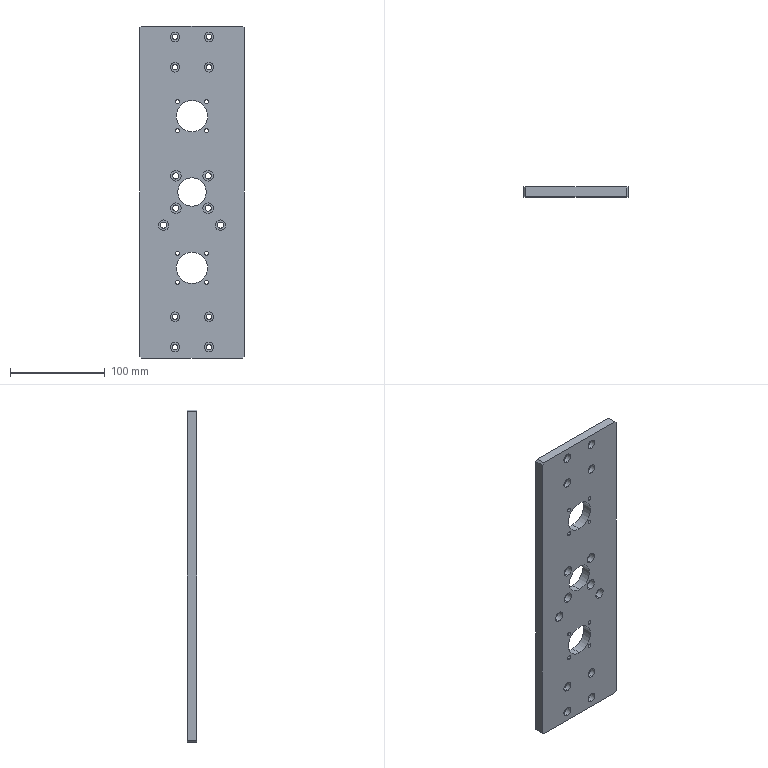Part | SolidWorks | features HoleWzd 4, ICE 2, Chamfer 1, Extrusion 1 | 1 solid | 102 faces | box 110 x 10 x 350 mm | volume 350704 mm3 | cylinder 78 | plane 24 | commonest cylinder face diameters 4.2 x16 5.5 x16 10 x16 6.6 x12 11 x12 33 x4